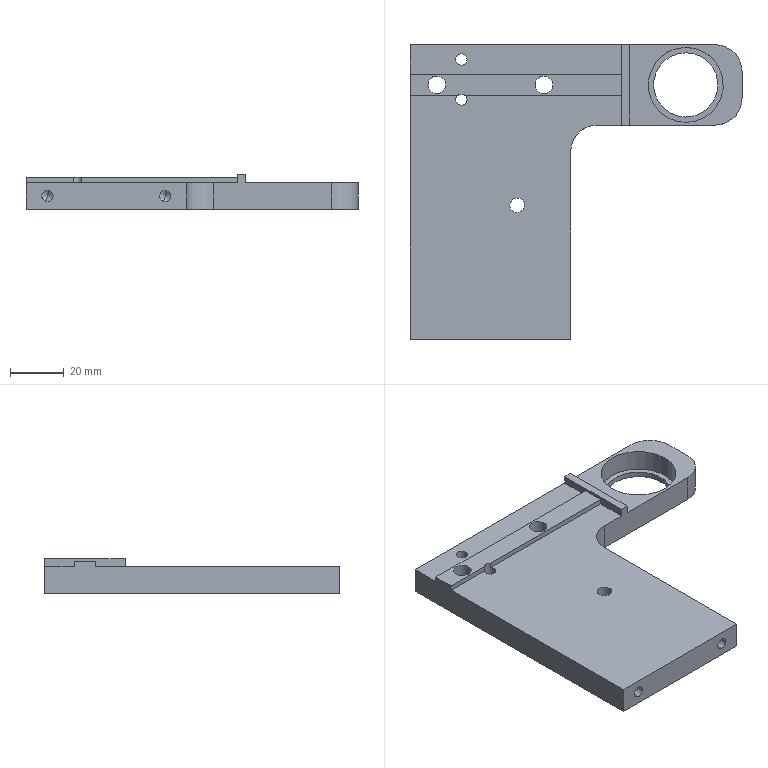Part | STEP file | 11-XSS102_PRT_33-1.PRT11 | 1 solid | 60 faces | box 124 x 110 x 13 mm | volume 77774 mm3 | cylinder 31 | plane 21 | cone 8 | commonest cylinder face diameters 4.2 x8 3.3 x4 6.6 x4 11 x4 20 x3 5.5 x2